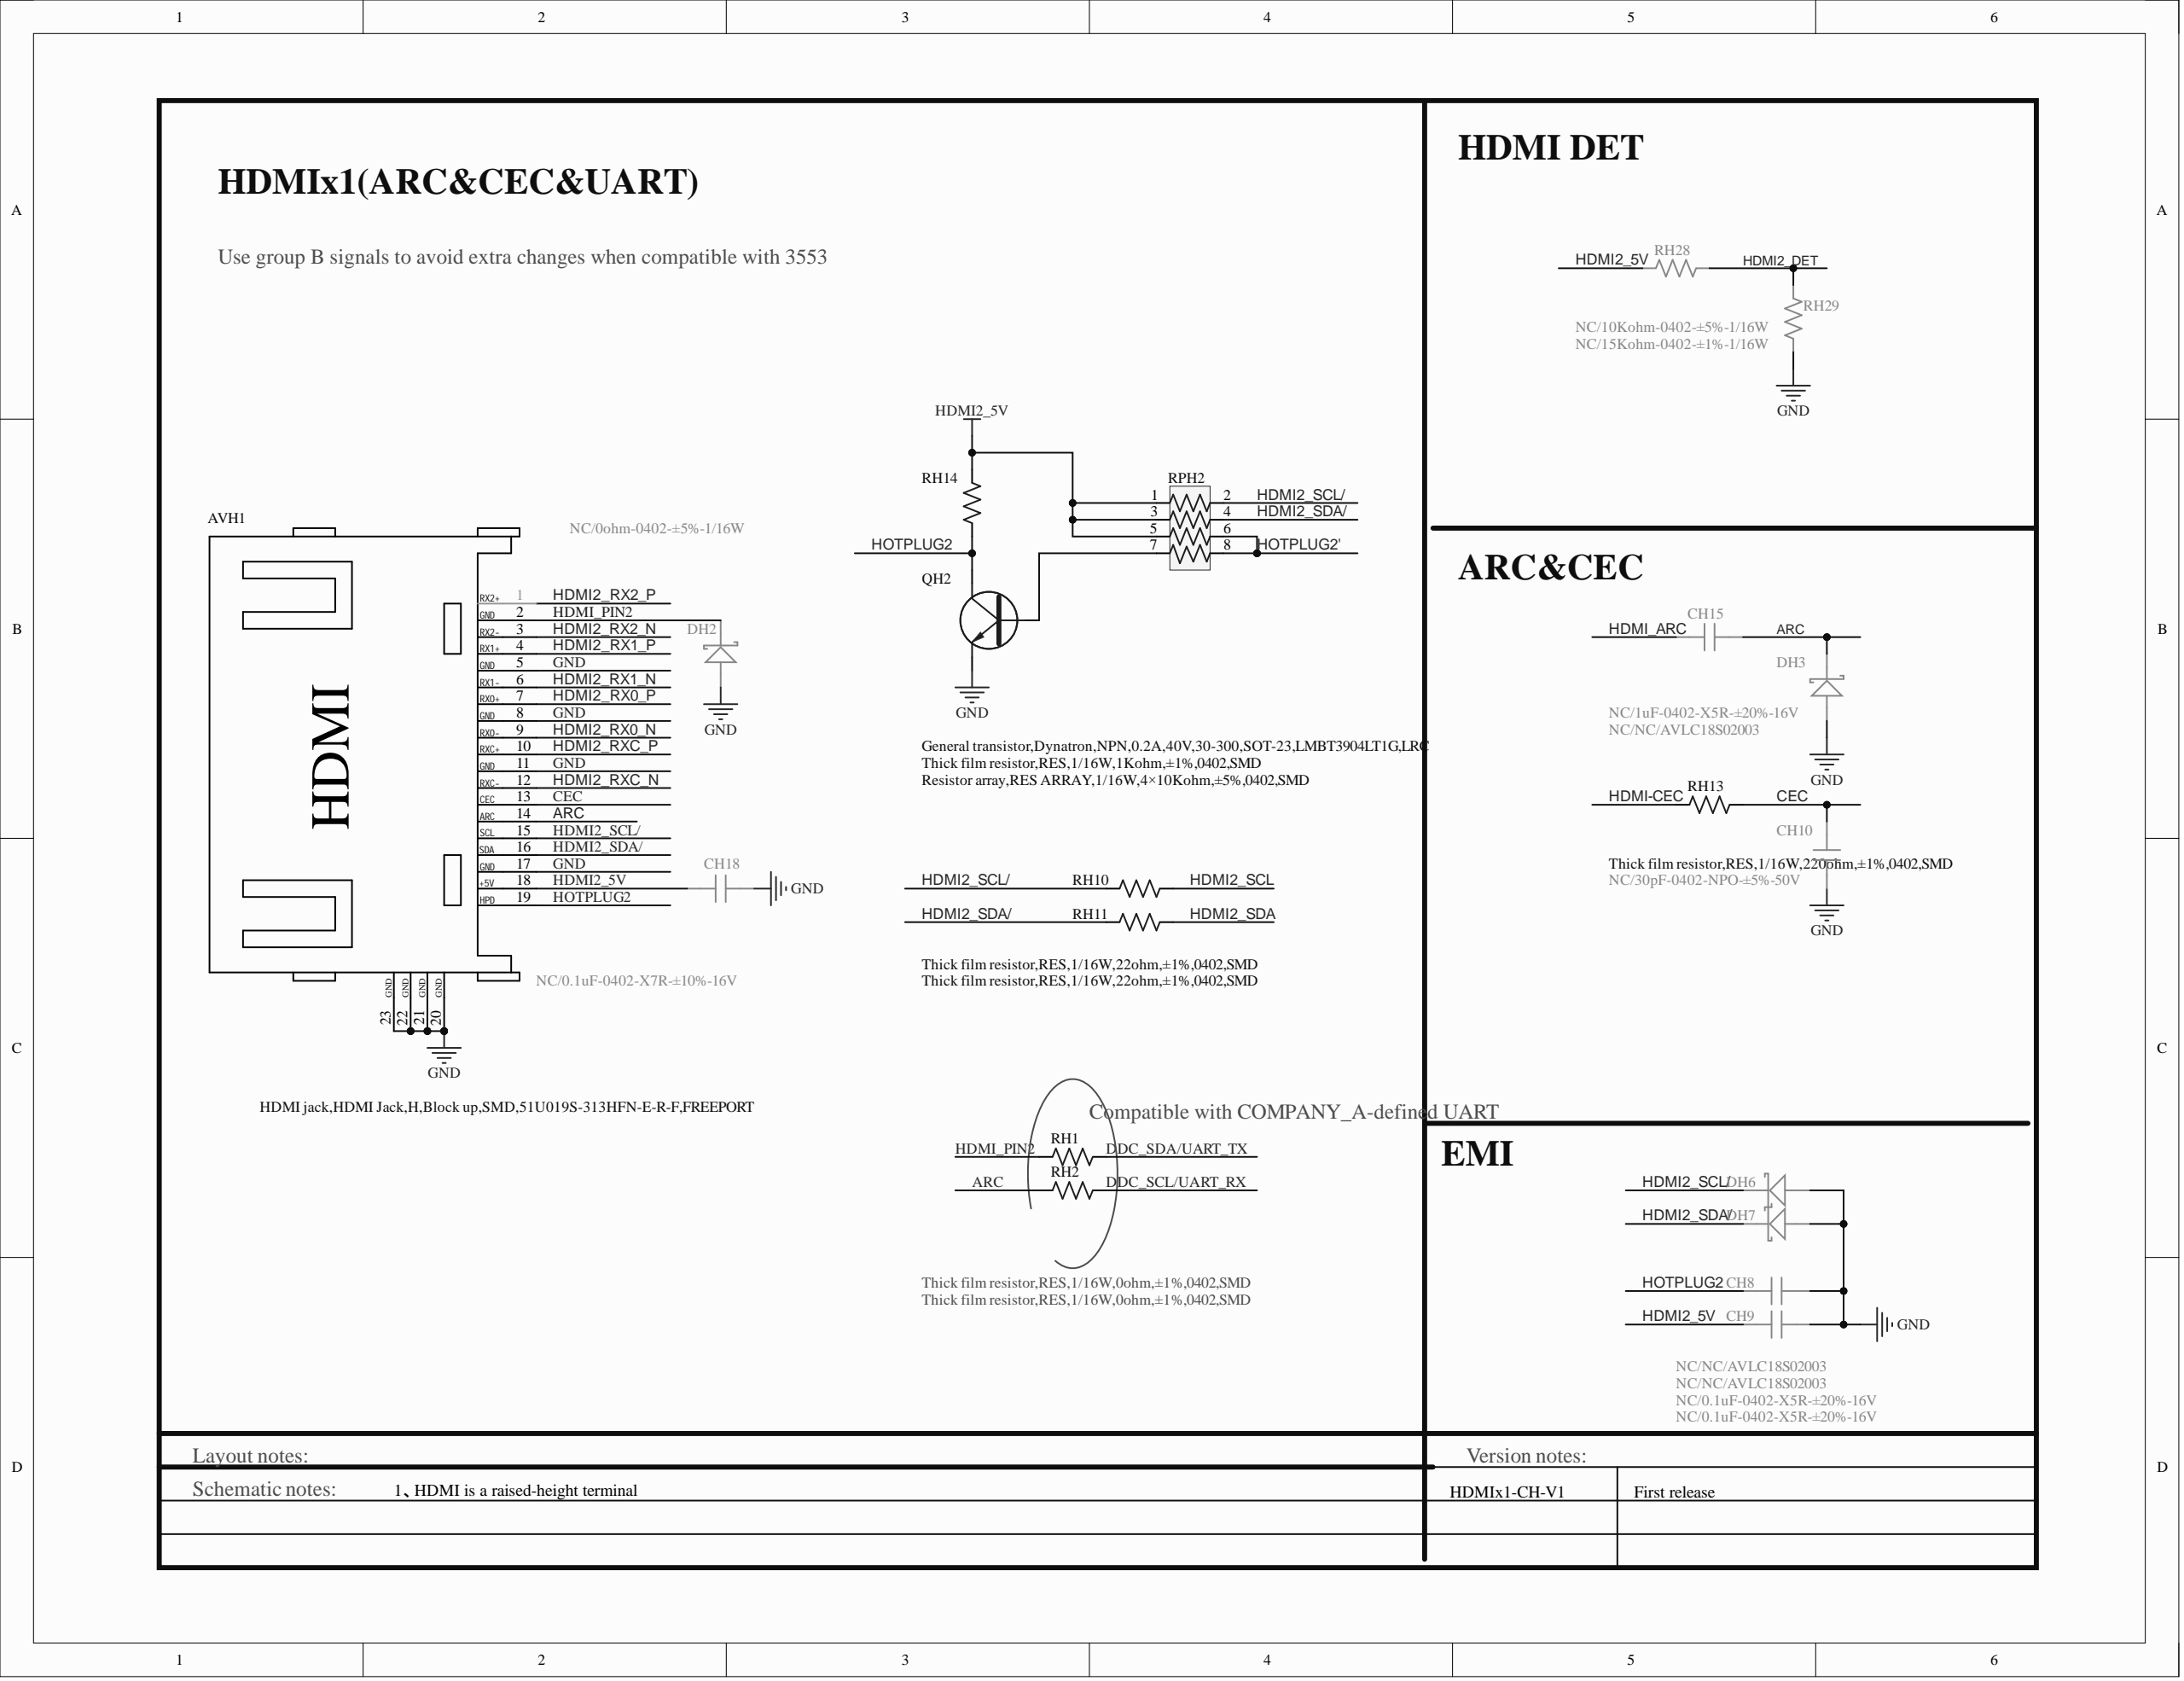Circuit board | Altium Designer | 719 parts | 352 nets | one sheet of the schematic
Parts on this sheet (reference | value | footprint):
AVH1 | HDMI jack,HDMI Jack,H,Block up,SMD,51U019S-313HFN-E-R-F,FREEPORT | HDMI-HS-11
CH8 | NC/0.1uF-0402-X5R-±20%-16V | C0402
CH9 | NC/0.1uF-0402-X5R-±20%-16V | C0402
CH10 | NC/30pF-0402-NPO-±5%-50V | C0402
CH15 | NC/1uF-0402-X5R-±20%-16V | C0402
CH18 | NC/0.1uF-0402-X7R-±10%-16V | C0402
DH2 | NC/0ohm-0402-±5%-1/16W | DIODE-S0402
DH3 | NC/NC/AVLC18S02003 | DIODE-S0402
DH6 | NC/NC/AVLC18S02003 | DIODE-S0402
DH7 | NC/NC/AVLC18S02003 | DIODE-S0402
QH2 | General transistor,Dynatron,NPN,0.2A,40V,30-300,SOT-23,LMBT3904LT1G,LRC | SOT-23
RH1 | Thick film resistor,RES,1/16W,0ohm,±1%,0402,SMD | R0402
RH2 | Thick film resistor,RES,1/16W,0ohm,±1%,0402,SMD | R0402
RH10 | Thick film resistor,RES,1/16W,22ohm,±1%,0402,SMD | R0402
RH11 | Thick film resistor,RES,1/16W,22ohm,±1%,0402,SMD | R0402
RH13 | Thick film resistor,RES,1/16W,220ohm,±1%,0402,SMD | R0402
RH14 | Thick film resistor,RES,1/16W,1Kohm,±1%,0402,SMD | R0402
RH28 | NC/10Kohm-0402-±5%-1/16W | R0402
RH29 | NC/15Kohm-0402-±1%-1/16W | R0402
RPH2 | Resistor array,RES ARRAY,1/16W,4×10Kohm,±5%,0402,SMD | RA0402
Nets of these parts (net: part-pin ...):
NetQH2_B: QH2-B RPH2-7
HOTPLUG2': RPH2-6 RPH2-8
HOTPLUG2: CH8-2 QH2-C RH14-1 AVH1-19
HDMI_PIN2: DH2-K RH1-1 AVH1-2
HDMI_ARC: CH15-2
HDMI-CEC: RH13-2
HDMI2_SDA/: DH7-K RH11-2 RPH2-4 AVH1-16
HDMI2_SDA: RH11-1
HDMI2_SCL/: DH6-K RH10-2 RPH2-2 AVH1-15
HDMI2_SCL: RH10-1
HDMI2_RXC_P: AVH1-10
HDMI2_RXC_N: AVH1-12
HDMI2_RX2_P: AVH1-1
HDMI2_RX2_N: AVH1-3
HDMI2_RX1_P: AVH1-4
HDMI2_RX1_N: AVH1-6
HDMI2_RX0_P: AVH1-7
HDMI2_RX0_N: AVH1-9
HDMI2_DET: RH28-1 RH29-1
HDMI2_5V: CH9-2 CH18-2 RH14-2 RH28-2 RPH2-1 RPH2-3 RPH2-5 AVH1-18
GND: CH8-1 CH9-1 CH10-1 CH18-1 DH2-A DH3-A DH6-A DH7-A QH2-E RH29-2 AVH1-5 AVH1-8 AVH1-11 AVH1-17 AVH1-20 AVH1-21 AVH1-22 AVH1-23
DDC_SDA/UART_TX: RH1-2
DDC_SCL/UART_RX: RH2-2
CEC: CH10-2 RH13-1 AVH1-13
ARC: CH15-1 DH3-K RH2-1 AVH1-14